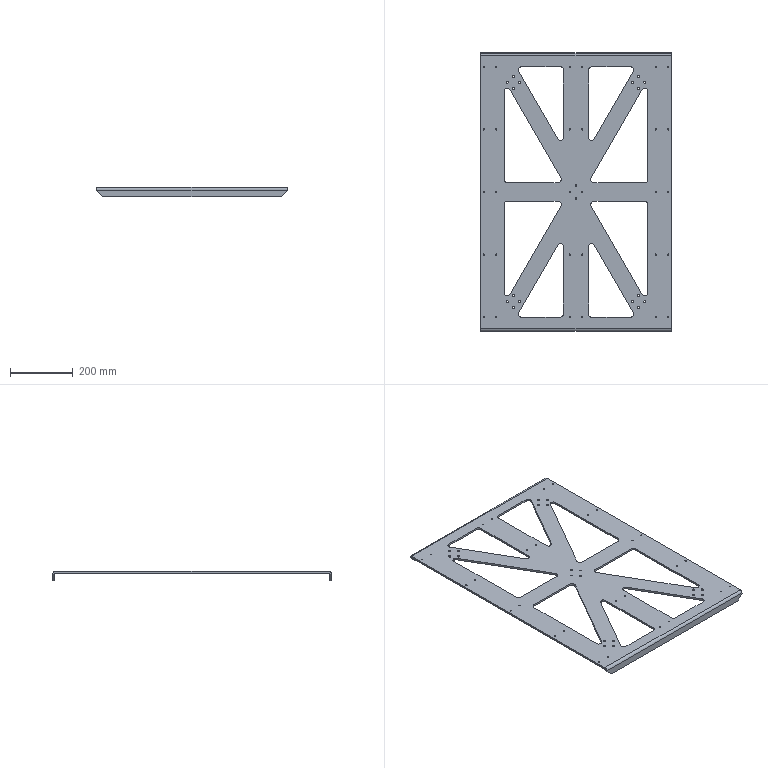Part | STEP file | LIFT.UPPER.PLATE.stp | 1 solid | 176 faces | box 610 x 890 x 30 mm | volume 2190669 mm3 | cylinder 106 | spline 50 | plane 20 | commonest cylinder face diameters 4 x60 20 x24 7 x16 6 x4 18 x2